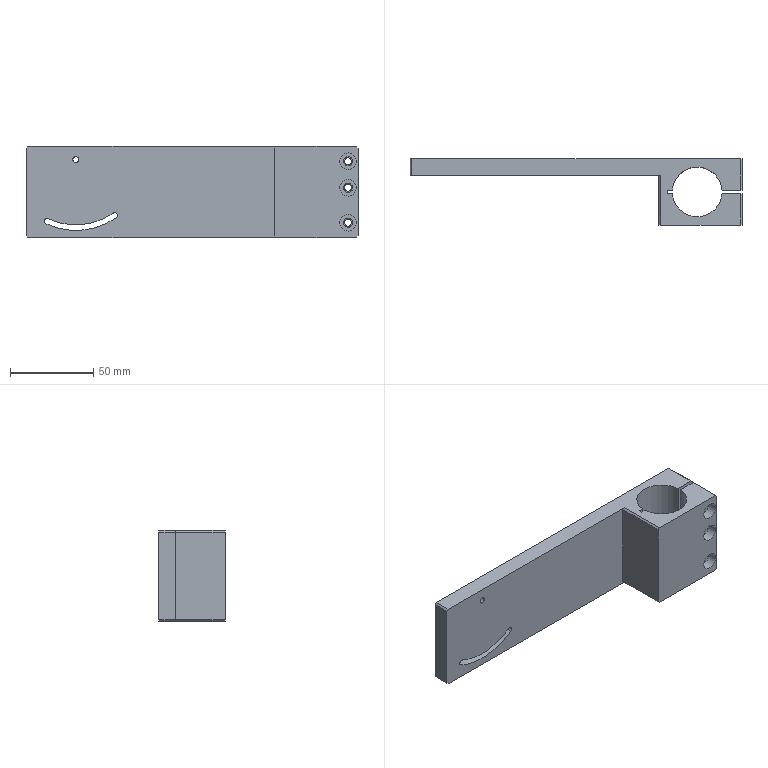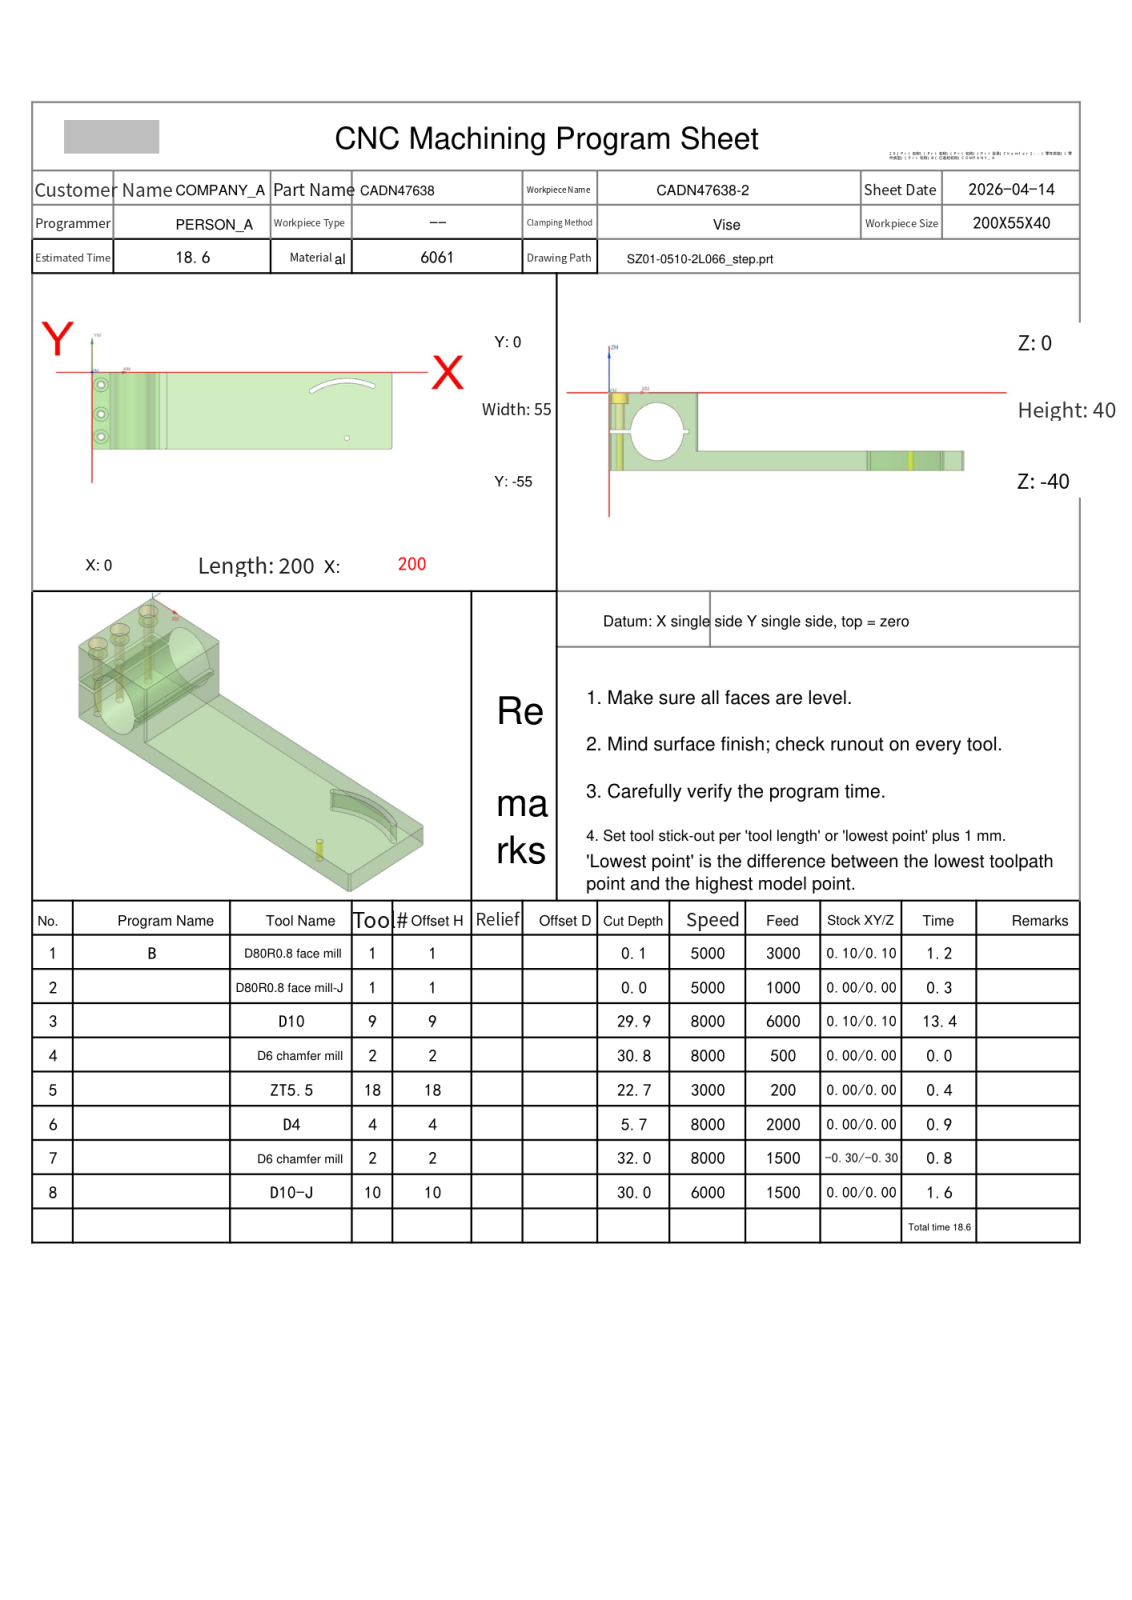NC program | NX | posted by the shop | part box 200 x 40 x 55 mm
Lines 113 to 1145 of 8619:
N3 T09 M06
(D10  D=10. R=0. H=09 ce=0.10 di=0.10)
(MAX_Z=14.8 MIN_Z=-29.9 Time=13.16M)
G00 G90 G54 X202.518 Y7.619 M03 S8000
G43 H09 Z14.8
M08
Z.902
G01 Z-.598 F6000.
X202.583 Y3.347
G02 X202.6 Y1.125 I-147.483 J-2.234
G01 Y-56.112
G02 X202.589 Y-57.94 I-147.5 J0.0
X202.296 Y-58.633 I-1. J.013
G01 X201.322 Y-59.607
G02 X200.616 Y-59.9 I-.707 J.707
G01 X198.47
G02 X197.571 Y-59. I.001 J.9
G01 Y-58.982
G03 X197.6 Y-56.112 I-142.471 J2.87
G01 Y1.124
G03 X197.572 Y3.92 I-142.5 J-.012
X196.573 Y4.9 I-1. J-.02
G01 X190.969
G03 X190.069 Y4. I.001 J-.9
G01 X190.07 Y3.981
G02 X190.1 Y1.124 I-134.97 J-2.869
G01 Y-56.112
G02 X190.071 Y-58.921 I-135. J0.0
X189.071 Y-59.9 I-1. J.021
G01 X183.467
G02 X182.568 Y-59. I.001 J.9
G01 Y-58.98
G03 X182.6 Y-56.112 I-127.468 J2.868
G01 Y1.123
G03 X182.569 Y3.922 I-127.5 J-.01
X181.57 Y4.9 I-1. J-.022
G01 X175.965
G03 X175.066 Y4. I.001 J-.9
G01 Y3.979
G02 X175.1 Y1.122 I-119.966 J-2.867
G01 Y-56.112
G02 X175.067 Y-58.924 I-120. J0.0
X174.068 Y-59.9 I-1. J.024
G01 X168.463
G02 X167.563 Y-59. I.001 J.9
G01 X167.564 Y-58.978
G03 X167.6 Y-56.112 I-112.464 J2.865
G01 Y1.122
G03 X167.565 Y3.925 I-112.5 J-.009
X166.565 Y4.9 I-1. J-.025
G01 X160.96
G03 X160.061 Y4. I.001 J-.9
G01 Y3.976
G02 X160.1 Y1.121 I-104.961 J-2.863
G01 Y-56.112
G02 X160.062 Y-58.927 I-105. J0.0
X159.063 Y-59.9 I-1. J.027
G01 X153.457
G02 X152.558 Y-59. I.001 J.9
G01 Y-58.974
G03 X152.6 Y-56.112 I-97.458 J2.862
G01 Y1.12
G03 X152.559 Y3.929 I-97.5 J-.008
X151.56 Y4.9 I-1. J-.029
G01 X145.954
G03 X145.054 Y4. I.001 J-.9
G01 X145.055 Y3.972
G02 X145.1 Y1.12 I-89.955 J-2.859
G01 Y-56.112
G02 X145.056 Y-58.932 I-90. J0.0
X144.057 Y-59.9 I-1. J.032
G01 X138.45
G02 X137.55 Y-59. I0.0 J.9
G01 X137.551 Y-58.969
G03 X137.6 Y-56.112 I-82.451 J2.857
G01 Y1.119
G03 X137.552 Y3.934 I-82.5 J-.007
X136.553 Y4.9 I-.999 J-.034
G01 X130.945
G03 X130.045 Y4. I.001 J-.9
G01 X130.046 Y3.966
G02 X130.1 Y1.119 I-74.946 J-2.854
G01 Y-56.112
G02 X130.047 Y-58.938 I-75. J0.0
X129.048 Y-59.9 I-.999 J.038
G01 X123.438
G02 X122.539 Y-59. I.001 J.9
G01 X122.54 Y-58.963
G03 X122.6 Y-56.112 I-67.44 J2.85
G01 Y1.118
G03 X122.541 Y3.942 I-67.5 J-.006
X121.542 Y4.9 I-.999 J-.042
G01 X115.931
G03 X115.032 Y4. I.001 J-.9
G01 Y3.958
G02 X115.1 Y1.117 I-59.932 J-2.845
G01 Y-56.112
G02 X115.033 Y-58.948 I-60. J0.0
X114.034 Y-59.9 I-.999 J.048
G01 X108.421
G02 X107.522 Y-59. I.001 J.9
G01 X107.523 Y-58.952
G03 X107.6 Y-56.112 I-52.423 J2.839
G01 Y1.117
G03 X107.523 Y3.954 I-52.5 J-.004
X106.525 Y4.9 I-.999 J-.054
G01 X100.909
G03 X100.009 Y4. I.001 J-.9
G01 X100.011 Y3.944
G02 X100.1 Y1.116 I-44.911 J-2.831
G01 Y-56.112
G02 X100.01 Y-58.964 I-45. J0.0
X99.012 Y-59.9 I-.998 J.064
G01 X93.391
G02 X92.491 Y-59. I.001 J.9
G01 X92.494 Y-58.933
G03 X92.6 Y-56.112 I-37.394 J2.82
G01 Y1.116
G03 X92.49 Y3.977 I-37.5 J-.003
X91.494 Y4.9 I-.997 J-.077
G01 X85.754
G03 X84.955 Y4.1 I.001 J-.8
G01 X84.958 Y4.023
G02 X85.1 Y1.115 I-29.858 J-2.91
G01 Y-56.112
G02 X84.961 Y-58.996 I-30. J0.0
X83.966 Y-59.9 I-.995 J.096
G01 X78.207
G02 X77.408 Y-59.1 I0.0 J.8
G01 X77.414 Y-58.998
G03 X77.6 Y-56.112 I-22.314 J2.885
G01 Y1.114
G03 X77.41 Y4.03 I-22.5 J-.002
X76.419 Y4.9 I-.992 J-.13
G01 X70.493
G03 X69.793 Y4.2 I0.0 J-.7
G01 X69.807 Y4.063
G02 X70.1 Y1.114 I-14.707 J-2.95
G01 Y-56.112
G02 X69.8 Y-59.099 I-15. J0.0
X68.82 Y-59.9 I-.98 J.199
G01 X62.546
G02 X61.946 Y-59.3 I0.0 J.6
X61.995 Y-59.064 I.6 J0.0
G03 X62.6 Y-56.112 I-6.895 J2.952
G01 Y1.112
G03 X61.818 Y4.446 I-7.5 J0.0
X61.101 Y4.985 I-.896 J-.445
G01 X52.197 Y6.591
X52.02 Y6.607
G03 X51.02 Y5.607 I0.0 J-1.
X51.312 Y4.9 I1. J0.0
G01 X55.1 Y1.112
Y-56.112
X51.312 Y-59.9
X48.112 Y-63.1
Z.902
G00 X202.518 Y7.619
Z.304
G01 Z-1.196
X202.583 Y3.347
G02 X202.6 Y1.125 I-147.483 J-2.234
G01 Y-56.112
G02 X202.589 Y-57.94 I-147.5 J0.0
X202.296 Y-58.633 I-1. J.013
G01 X201.322 Y-59.607
G02 X200.616 Y-59.9 I-.707 J.707
G01 X198.47
G02 X197.571 Y-59. I.001 J.9
G01 Y-58.982
G03 X197.6 Y-56.112 I-142.471 J2.87
G01 Y1.124
G03 X197.572 Y3.92 I-142.5 J-.012
X196.573 Y4.9 I-1. J-.02
G01 X190.969
G03 X190.069 Y4. I.001 J-.9
G01 X190.07 Y3.981
G02 X190.1 Y1.124 I-134.97 J-2.869
G01 Y-56.112
G02 X190.071 Y-58.921 I-135. J0.0
X189.071 Y-59.9 I-1. J.021
G01 X183.467
G02 X182.568 Y-59. I.001 J.9
G01 Y-58.98
G03 X182.6 Y-56.112 I-127.468 J2.868
G01 Y1.123
G03 X182.569 Y3.922 I-127.5 J-.01
X181.57 Y4.9 I-1. J-.022
G01 X175.965
G03 X175.066 Y4. I.001 J-.9
G01 Y3.979
G02 X175.1 Y1.122 I-119.966 J-2.867
G01 Y-56.112
G02 X175.067 Y-58.924 I-120. J0.0
X174.068 Y-59.9 I-1. J.024
G01 X168.463
G02 X167.563 Y-59. I.001 J.9
G01 X167.564 Y-58.978
G03 X167.6 Y-56.112 I-112.464 J2.865
G01 Y1.122
G03 X167.565 Y3.925 I-112.5 J-.009
X166.565 Y4.9 I-1. J-.025
G01 X160.96
G03 X160.061 Y4. I.001 J-.9
G01 Y3.976
G02 X160.1 Y1.121 I-104.961 J-2.863
G01 Y-56.112
G02 X160.062 Y-58.927 I-105. J0.0
X159.063 Y-59.9 I-1. J.027
G01 X153.457
G02 X152.558 Y-59. I.001 J.9
G01 Y-58.974
G03 X152.6 Y-56.112 I-97.458 J2.862
G01 Y1.12
G03 X152.559 Y3.929 I-97.5 J-.008
X151.56 Y4.9 I-1. J-.029
G01 X145.954
G03 X145.054 Y4. I.001 J-.9
G01 X145.055 Y3.972
G02 X145.1 Y1.12 I-89.955 J-2.859
G01 Y-56.112
G02 X145.056 Y-58.932 I-90. J0.0
X144.057 Y-59.9 I-1. J.032
G01 X138.45
G02 X137.55 Y-59. I0.0 J.9
G01 X137.551 Y-58.969
G03 X137.6 Y-56.112 I-82.451 J2.857
G01 Y1.119
G03 X137.552 Y3.934 I-82.5 J-.007
X136.553 Y4.9 I-.999 J-.034
G01 X130.945
G03 X130.045 Y4. I.001 J-.9
G01 X130.046 Y3.966
G02 X130.1 Y1.119 I-74.946 J-2.854
G01 Y-56.112
G02 X130.047 Y-58.938 I-75. J0.0
X129.048 Y-59.9 I-.999 J.038
G01 X123.438
G02 X122.539 Y-59. I.001 J.9
G01 X122.54 Y-58.963
G03 X122.6 Y-56.112 I-67.44 J2.85
G01 Y1.118
G03 X122.541 Y3.942 I-67.5 J-.006
X121.542 Y4.9 I-.999 J-.042
G01 X115.931
G03 X115.032 Y4. I.001 J-.9
G01 Y3.958
G02 X115.1 Y1.117 I-59.932 J-2.845
G01 Y-56.112
G02 X115.033 Y-58.948 I-60. J0.0
X114.034 Y-59.9 I-.999 J.048
G01 X108.421
G02 X107.522 Y-59. I.001 J.9
G01 X107.523 Y-58.952
G03 X107.6 Y-56.112 I-52.423 J2.839
G01 Y1.117
G03 X107.523 Y3.954 I-52.5 J-.004
X106.525 Y4.9 I-.999 J-.054
G01 X100.909
G03 X100.009 Y4. I.001 J-.9
G01 X100.011 Y3.944
G02 X100.1 Y1.116 I-44.911 J-2.831
G01 Y-56.112
G02 X100.01 Y-58.964 I-45. J0.0
X99.012 Y-59.9 I-.998 J.064
G01 X93.391
G02 X92.491 Y-59. I.001 J.9
G01 X92.494 Y-58.933
G03 X92.6 Y-56.112 I-37.394 J2.82
G01 Y1.116
G03 X92.49 Y3.977 I-37.5 J-.003
X91.494 Y4.9 I-.997 J-.077
G01 X85.754
G03 X84.955 Y4.1 I.001 J-.8
G01 X84.958 Y4.023
G02 X85.1 Y1.115 I-29.858 J-2.91
G01 Y-56.112
G02 X84.961 Y-58.996 I-30. J0.0
X83.966 Y-59.9 I-.995 J.096
G01 X78.207
G02 X77.408 Y-59.1 I0.0 J.8
G01 X77.414 Y-58.998
G03 X77.6 Y-56.112 I-22.314 J2.885
G01 Y1.114
G03 X77.41 Y4.03 I-22.5 J-.002
X76.419 Y4.9 I-.992 J-.13
G01 X70.493
G03 X69.793 Y4.2 I0.0 J-.7
G01 X69.807 Y4.063
G02 X70.1 Y1.114 I-14.707 J-2.95
G01 Y-56.112
G02 X69.8 Y-59.099 I-15. J0.0
X68.82 Y-59.9 I-.98 J.199
G01 X62.546
G02 X61.946 Y-59.3 I0.0 J.6
X61.995 Y-59.064 I.6 J0.0
G03 X62.6 Y-56.112 I-6.895 J2.952
G01 Y1.112
G03 X61.818 Y4.446 I-7.5 J0.0
X61.101 Y4.985 I-.896 J-.445
G01 X52.197 Y6.591
X52.02 Y6.607
G03 X51.02 Y5.607 I0.0 J-1.
X51.312 Y4.9 I1. J0.0
G01 X55.1 Y1.112
Y-56.112
X51.312 Y-59.9
X48.112 Y-63.1
Z.304
G00 X202.518 Y7.619
Z-.294
G01 Z-1.794
X202.583 Y3.347
G02 X202.6 Y1.125 I-147.483 J-2.234
G01 Y-56.112
G02 X202.589 Y-57.94 I-147.5 J0.0
X202.296 Y-58.633 I-1. J.013
G01 X201.322 Y-59.607
G02 X200.616 Y-59.9 I-.707 J.707
G01 X198.47
G02 X197.571 Y-59. I.001 J.9
G01 Y-58.982
G03 X197.6 Y-56.112 I-142.471 J2.87
G01 Y1.124
G03 X197.572 Y3.92 I-142.5 J-.012
X196.573 Y4.9 I-1. J-.02
G01 X190.969
G03 X190.069 Y4. I.001 J-.9
G01 X190.07 Y3.981
G02 X190.1 Y1.124 I-134.97 J-2.869
G01 Y-56.112
G02 X190.071 Y-58.921 I-135. J0.0
X189.071 Y-59.9 I-1. J.021
G01 X183.467
G02 X182.568 Y-59. I.001 J.9
G01 Y-58.98
G03 X182.6 Y-56.112 I-127.468 J2.868
G01 Y1.123
G03 X182.569 Y3.922 I-127.5 J-.01
X181.57 Y4.9 I-1. J-.022
G01 X175.965
G03 X175.066 Y4. I.001 J-.9
G01 Y3.979
G02 X175.1 Y1.122 I-119.966 J-2.867
G01 Y-56.112
G02 X175.067 Y-58.924 I-120. J0.0
X174.068 Y-59.9 I-1. J.024
G01 X168.463
G02 X167.563 Y-59. I.001 J.9
G01 X167.564 Y-58.978
G03 X167.6 Y-56.112 I-112.464 J2.865
G01 Y1.122
G03 X167.565 Y3.925 I-112.5 J-.009
X166.565 Y4.9 I-1. J-.025
G01 X160.96
G03 X160.061 Y4. I.001 J-.9
G01 Y3.976
G02 X160.1 Y1.121 I-104.961 J-2.863
G01 Y-56.112
G02 X160.062 Y-58.927 I-105. J0.0
X159.063 Y-59.9 I-1. J.027
G01 X153.457
G02 X152.558 Y-59. I.001 J.9
G01 Y-58.974
G03 X152.6 Y-56.112 I-97.458 J2.862
G01 Y1.12
G03 X152.559 Y3.929 I-97.5 J-.008
X151.56 Y4.9 I-1. J-.029
G01 X145.954
G03 X145.054 Y4. I.001 J-.9
G01 X145.055 Y3.972
G02 X145.1 Y1.12 I-89.955 J-2.859
G01 Y-56.112
G02 X145.056 Y-58.932 I-90. J0.0
X144.057 Y-59.9 I-1. J.032
G01 X138.45
G02 X137.55 Y-59. I0.0 J.9
G01 X137.551 Y-58.969
G03 X137.6 Y-56.112 I-82.451 J2.857
G01 Y1.119
G03 X137.552 Y3.934 I-82.5 J-.007
X136.553 Y4.9 I-.999 J-.034
G01 X130.945
G03 X130.045 Y4. I.001 J-.9
G01 X130.046 Y3.966
G02 X130.1 Y1.119 I-74.946 J-2.854
G01 Y-56.112
G02 X130.047 Y-58.938 I-75. J0.0
X129.048 Y-59.9 I-.999 J.038
G01 X123.438
G02 X122.539 Y-59. I.001 J.9
G01 X122.54 Y-58.963
G03 X122.6 Y-56.112 I-67.44 J2.85
G01 Y1.118
G03 X122.541 Y3.942 I-67.5 J-.006
X121.542 Y4.9 I-.999 J-.042
G01 X115.931
G03 X115.032 Y4. I.001 J-.9
G01 Y3.958
G02 X115.1 Y1.117 I-59.932 J-2.845
G01 Y-56.112
G02 X115.033 Y-58.948 I-60. J0.0
X114.034 Y-59.9 I-.999 J.048
G01 X108.421
G02 X107.522 Y-59. I.001 J.9
G01 X107.523 Y-58.952
G03 X107.6 Y-56.112 I-52.423 J2.839
G01 Y1.117
G03 X107.523 Y3.954 I-52.5 J-.004
X106.525 Y4.9 I-.999 J-.054
G01 X100.909
G03 X100.009 Y4. I.001 J-.9
G01 X100.011 Y3.944
G02 X100.1 Y1.116 I-44.911 J-2.831
G01 Y-56.112
G02 X100.01 Y-58.964 I-45. J0.0
X99.012 Y-59.9 I-.998 J.064
G01 X93.391
G02 X92.491 Y-59. I.001 J.9
G01 X92.494 Y-58.933
G03 X92.6 Y-56.112 I-37.394 J2.82
G01 Y1.116
G03 X92.49 Y3.977 I-37.5 J-.003
X91.494 Y4.9 I-.997 J-.077
G01 X85.754
G03 X84.955 Y4.1 I.001 J-.8
G01 X84.958 Y4.023
G02 X85.1 Y1.115 I-29.858 J-2.91
G01 Y-56.112
G02 X84.961 Y-58.996 I-30. J0.0
X83.966 Y-59.9 I-.995 J.096
G01 X78.207
G02 X77.408 Y-59.1 I0.0 J.8
G01 X77.414 Y-58.998
G03 X77.6 Y-56.112 I-22.314 J2.885
G01 Y1.114
G03 X77.41 Y4.03 I-22.5 J-.002
X76.419 Y4.9 I-.992 J-.13
G01 X70.493
G03 X69.793 Y4.2 I0.0 J-.7
G01 X69.807 Y4.063
G02 X70.1 Y1.114 I-14.707 J-2.95
G01 Y-56.112
G02 X69.8 Y-59.099 I-15. J0.0
X68.82 Y-59.9 I-.98 J.199
G01 X62.546
G02 X61.946 Y-59.3 I0.0 J.6
X61.995 Y-59.064 I.6 J0.0
G03 X62.6 Y-56.112 I-6.895 J2.952
G01 Y1.112
G03 X61.818 Y4.446 I-7.5 J0.0
X61.101 Y4.985 I-.896 J-.445
G01 X52.197 Y6.591
X52.02 Y6.607
G03 X51.02 Y5.607 I0.0 J-1.
X51.312 Y4.9 I1. J0.0
G01 X55.1 Y1.112
Y-56.112
X51.312 Y-59.9
X48.112 Y-63.1
Z-.294
G00 X202.518 Y7.619
Z-.892
G01 Z-2.392
X202.583 Y3.347
G02 X202.6 Y1.125 I-147.483 J-2.234
G01 Y-56.112
G02 X202.589 Y-57.94 I-147.5 J0.0
X202.296 Y-58.633 I-1. J.013
G01 X201.322 Y-59.607
G02 X200.616 Y-59.9 I-.707 J.707
G01 X198.47
G02 X197.571 Y-59. I.001 J.9
G01 Y-58.982
G03 X197.6 Y-56.112 I-142.471 J2.87
G01 Y1.124
G03 X197.572 Y3.92 I-142.5 J-.012
X196.573 Y4.9 I-1. J-.02
G01 X190.969
G03 X190.069 Y4. I.001 J-.9
G01 X190.07 Y3.981
G02 X190.1 Y1.124 I-134.97 J-2.869
G01 Y-56.112
G02 X190.071 Y-58.921 I-135. J0.0
X189.071 Y-59.9 I-1. J.021
G01 X183.467
G02 X182.568 Y-59. I.001 J.9
G01 Y-58.98
G03 X182.6 Y-56.112 I-127.468 J2.868
G01 Y1.123
G03 X182.569 Y3.922 I-127.5 J-.01
X181.57 Y4.9 I-1. J-.022
G01 X175.965
G03 X175.066 Y4. I.001 J-.9
G01 Y3.979
G02 X175.1 Y1.122 I-119.966 J-2.867
G01 Y-56.112
G02 X175.067 Y-58.924 I-120. J0.0
X174.068 Y-59.9 I-1. J.024
G01 X168.463
G02 X167.563 Y-59. I.001 J.9
G01 X167.564 Y-58.978
G03 X167.6 Y-56.112 I-112.464 J2.865
G01 Y1.122
G03 X167.565 Y3.925 I-112.5 J-.009
X166.565 Y4.9 I-1. J-.025
G01 X160.96
G03 X160.061 Y4. I.001 J-.9
G01 Y3.976
G02 X160.1 Y1.121 I-104.961 J-2.863
G01 Y-56.112
G02 X160.062 Y-58.927 I-105. J0.0
X159.063 Y-59.9 I-1. J.027
G01 X153.457
G02 X152.558 Y-59. I.001 J.9
G01 Y-58.974
G03 X152.6 Y-56.112 I-97.458 J2.862
G01 Y1.12
G03 X152.559 Y3.929 I-97.5 J-.008
X151.56 Y4.9 I-1. J-.029
G01 X145.954
G03 X145.054 Y4. I.001 J-.9
G01 X145.055 Y3.972
G02 X145.1 Y1.12 I-89.955 J-2.859
G01 Y-56.112
G02 X145.056 Y-58.932 I-90. J0.0
X144.057 Y-59.9 I-1. J.032
G01 X138.45
G02 X137.55 Y-59. I0.0 J.9
G01 X137.551 Y-58.969
G03 X137.6 Y-56.112 I-82.451 J2.857
G01 Y1.119
G03 X137.552 Y3.934 I-82.5 J-.007
X136.553 Y4.9 I-.999 J-.034
G01 X130.945
G03 X130.045 Y4. I.001 J-.9
G01 X130.046 Y3.966
G02 X130.1 Y1.119 I-74.946 J-2.854
G01 Y-56.112
G02 X130.047 Y-58.938 I-75. J0.0
X129.048 Y-59.9 I-.999 J.038
G01 X123.438
G02 X122.539 Y-59. I.001 J.9
G01 X122.54 Y-58.963
G03 X122.6 Y-56.112 I-67.44 J2.85
G01 Y1.118
G03 X122.541 Y3.942 I-67.5 J-.006
X121.542 Y4.9 I-.999 J-.042
G01 X115.931
G03 X115.032 Y4. I.001 J-.9
G01 Y3.958
G02 X115.1 Y1.117 I-59.932 J-2.845
G01 Y-56.112
G02 X115.033 Y-58.948 I-60. J0.0
X114.034 Y-59.9 I-.999 J.048
G01 X108.421
G02 X107.522 Y-59. I.001 J.9
G01 X107.523 Y-58.952
G03 X107.6 Y-56.112 I-52.423 J2.839
G01 Y1.117
G03 X107.523 Y3.954 I-52.5 J-.004
X106.525 Y4.9 I-.999 J-.054
G01 X100.909
G03 X100.009 Y4. I.001 J-.9
G01 X100.011 Y3.944
G02 X100.1 Y1.116 I-44.911 J-2.831
G01 Y-56.112
G02 X100.01 Y-58.964 I-45. J0.0
X99.012 Y-59.9 I-.998 J.064
G01 X93.391
G02 X92.491 Y-59. I.001 J.9
G01 X92.494 Y-58.933
G03 X92.6 Y-56.112 I-37.394 J2.82
G01 Y1.116
G03 X92.49 Y3.977 I-37.5 J-.003
X91.494 Y4.9 I-.997 J-.077
G01 X85.754
G03 X84.955 Y4.1 I.001 J-.8
G01 X84.958 Y4.023
G02 X85.1 Y1.115 I-29.858 J-2.91
G01 Y-56.112
G02 X84.961 Y-58.996 I-30. J0.0
X83.966 Y-59.9 I-.995 J.096
G01 X78.207
G02 X77.408 Y-59.1 I0.0 J.8
G01 X77.414 Y-58.998
G03 X77.6 Y-56.112 I-22.314 J2.885
G01 Y1.114
G03 X77.41 Y4.03 I-22.5 J-.002
X76.419 Y4.9 I-.992 J-.13
G01 X70.493
G03 X69.793 Y4.2 I0.0 J-.7
G01 X69.807 Y4.063
G02 X70.1 Y1.114 I-14.707 J-2.95
G01 Y-56.112
G02 X69.8 Y-59.099 I-15. J0.0
X68.82 Y-59.9 I-.98 J.199
G01 X62.546
G02 X61.946 Y-59.3 I0.0 J.6
X61.995 Y-59.064 I.6 J0.0
G03 X62.6 Y-56.112 I-6.895 J2.952
G01 Y1.112
G03 X61.818 Y4.446 I-7.5 J0.0
X61.101 Y4.985 I-.896 J-.445
G01 X52.197 Y6.591
X52.02 Y6.607
G03 X51.02 Y5.607 I0.0 J-1.
X51.312 Y4.9 I1. J0.0
G01 X55.1 Y1.112
Y-56.112
X51.312 Y-59.9
X48.112 Y-63.1
Z-.892
G00 X202.518 Y7.619
Z-1.49
G01 Z-2.99
X202.583 Y3.347
G02 X202.6 Y1.125 I-147.483 J-2.234
G01 Y-56.112
G02 X202.589 Y-57.94 I-147.5 J0.0
X202.296 Y-58.633 I-1. J.013
G01 X201.322 Y-59.607
G02 X200.616 Y-59.9 I-.707 J.707
G01 X198.47
G02 X197.571 Y-59. I.001 J.9
G01 Y-58.982
G03 X197.6 Y-56.112 I-142.471 J2.87
G01 Y1.124
G03 X197.572 Y3.92 I-142.5 J-.012
X196.573 Y4.9 I-1. J-.02
G01 X190.969
G03 X190.069 Y4. I.001 J-.9
G01 X190.07 Y3.981
G02 X190.1 Y1.124 I-134.97 J-2.869
G01 Y-56.112
G02 X190.071 Y-58.921 I-135. J0.0
X189.071 Y-59.9 I-1. J.021
G01 X183.467
G02 X182.568 Y-59. I.001 J.9
G01 Y-58.98
G03 X182.6 Y-56.112 I-127.468 J2.868
G01 Y1.123
G03 X182.569 Y3.922 I-127.5 J-.01
X181.57 Y4.9 I-1. J-.022
G01 X175.965
G03 X175.066 Y4. I.001 J-.9
G01 Y3.979
G02 X175.1 Y1.122 I-119.966 J-2.867
G01 Y-56.112
G02 X175.067 Y-58.924 I-120. J0.0
X174.068 Y-59.9 I-1. J.024
G01 X168.463
G02 X167.563 Y-59. I.001 J.9
G01 X167.564 Y-58.978
G03 X167.6 Y-56.112 I-112.464 J2.865
G01 Y1.122
G03 X167.565 Y3.925 I-112.5 J-.009
X166.565 Y4.9 I-1. J-.025
G01 X160.96
G03 X160.061 Y4. I.001 J-.9
G01 Y3.976
G02 X160.1 Y1.121 I-104.961 J-2.863
G01 Y-56.112
G02 X160.062 Y-58.927 I-105. J0.0
X159.063 Y-59.9 I-1. J.027
G01 X153.457
G02 X152.558 Y-59. I.001 J.9
G01 Y-58.974
G03 X152.6 Y-56.112 I-97.458 J2.862
G01 Y1.12
G03 X152.559 Y3.929 I-97.5 J-.008
X151.56 Y4.9 I-1. J-.029
G01 X145.954
G03 X145.054 Y4. I.001 J-.9
G01 X145.055 Y3.972
G02 X145.1 Y1.12 I-89.955 J-2.859
G01 Y-56.112
G02 X145.056 Y-58.932 I-90. J0.0
X144.057 Y-59.9 I-1. J.032
G01 X138.45
G02 X137.55 Y-59. I0.0 J.9
G01 X137.551 Y-58.969
G03 X137.6 Y-56.112 I-82.451 J2.857
G01 Y1.119
G03 X137.552 Y3.934 I-82.5 J-.007
X136.553 Y4.9 I-.999 J-.034
G01 X130.945
G03 X130.045 Y4. I.001 J-.9
G01 X130.046 Y3.966
G02 X130.1 Y1.119 I-74.946 J-2.854
G01 Y-56.112
G02 X130.047 Y-58.938 I-75. J0.0
X129.048 Y-59.9 I-.999 J.038
G01 X123.438
G02 X122.539 Y-59. I.001 J.9
G01 X122.54 Y-58.963
G03 X122.6 Y-56.112 I-67.44 J2.85
G01 Y1.118
G03 X122.541 Y3.942 I-67.5 J-.006
X121.542 Y4.9 I-.999 J-.042
G01 X115.931
G03 X115.032 Y4. I.001 J-.9
G01 Y3.958
G02 X115.1 Y1.117 I-59.932 J-2.845
G01 Y-56.112
G02 X115.033 Y-58.948 I-60. J0.0
X114.034 Y-59.9 I-.999 J.048
G01 X108.421
G02 X107.522 Y-59. I.001 J.9
G01 X107.523 Y-58.952
G03 X107.6 Y-56.112 I-52.423 J2.839
G01 Y1.117
G03 X107.523 Y3.954 I-52.5 J-.004
X106.525 Y4.9 I-.999 J-.054
G01 X100.909
G03 X100.009 Y4. I.001 J-.9
G01 X100.011 Y3.944
G02 X100.1 Y1.116 I-44.911 J-2.831
G01 Y-56.112
G02 X100.01 Y-58.964 I-45. J0.0
X99.012 Y-59.9 I-.998 J.064
G01 X93.391
G02 X92.491 Y-59. I.001 J.9
G01 X92.494 Y-58.933
G03 X92.6 Y-56.112 I-37.394 J2.82
G01 Y1.116
G03 X92.49 Y3.977 I-37.5 J-.003
X91.494 Y4.9 I-.997 J-.077
G01 X85.754
G03 X84.955 Y4.1 I.001 J-.8
G01 X84.958 Y4.023
G02 X85.1 Y1.115 I-29.858 J-2.91
G01 Y-56.112
G02 X84.961 Y-58.996 I-30. J0.0
X83.966 Y-59.9 I-.995 J.096
G01 X78.207
G02 X77.408 Y-59.1 I0.0 J.8
G01 X77.414 Y-58.998
G03 X77.6 Y-56.112 I-22.314 J2.885
G01 Y1.114
G03 X77.41 Y4.03 I-22.5 J-.002
X76.419 Y4.9 I-.992 J-.13
G01 X70.493
G03 X69.793 Y4.2 I0.0 J-.7
G01 X69.807 Y4.063
G02 X70.1 Y1.114 I-14.707 J-2.95
G01 Y-56.112
G02 X69.8 Y-59.099 I-15. J0.0
X68.82 Y-59.9 I-.98 J.199
G01 X62.546
G02 X61.946 Y-59.3 I0.0 J.6
X61.995 Y-59.064 I.6 J0.0
G03 X62.6 Y-56.112 I-6.895 J2.952
G01 Y1.112
G03 X61.818 Y4.446 I-7.5 J0.0
X61.101 Y4.985 I-.896 J-.445
G01 X52.197 Y6.591
X52.02 Y6.607
G03 X51.02 Y5.607 I0.0 J-1.
X51.312 Y4.9 I1. J0.0
G01 X55.1 Y1.112
Y-56.112
X51.312 Y-59.9
X48.112 Y-63.1
Z-1.49
G00 X202.518 Y7.619
Z-2.088
G01 Z-3.588
X202.583 Y3.347
G02 X202.6 Y1.125 I-147.483 J-2.234
G01 Y-56.112
G02 X202.589 Y-57.94 I-147.5 J0.0
X202.296 Y-58.633 I-1. J.013
G01 X201.322 Y-59.607
G02 X200.616 Y-59.9 I-.707 J.707
G01 X198.47
G02 X197.571 Y-59. I.001 J.9
G01 Y-58.982
G03 X197.6 Y-56.112 I-142.471 J2.87
G01 Y1.124
G03 X197.572 Y3.92 I-142.5 J-.012
X196.573 Y4.9 I-1. J-.02
G01 X190.969
G03 X190.069 Y4. I.001 J-.9
G01 X190.07 Y3.981
G02 X190.1 Y1.124 I-134.97 J-2.869
G01 Y-56.112
G02 X190.071 Y-58.921 I-135. J0.0
X189.071 Y-59.9 I-1. J.021
G01 X183.467
G02 X182.568 Y-59. I.001 J.9
G01 Y-58.98
G03 X182.6 Y-56.112 I-127.468 J2.868
G01 Y1.123
G03 X182.569 Y3.922 I-127.5 J-.01
X181.57 Y4.9 I-1. J-.022
G01 X175.965
G03 X175.066 Y4. I.001 J-.9
G01 Y3.979
G02 X175.1 Y1.122 I-119.966 J-2.867
G01 Y-56.112
G02 X175.067 Y-58.924 I-120. J0.0
X174.068 Y-59.9 I-1. J.024
G01 X168.463
G02 X167.563 Y-59. I.001 J.9
G01 X167.564 Y-58.978
G03 X167.6 Y-56.112 I-112.464 J2.865
G01 Y1.122
G03 X167.565 Y3.925 I-112.5 J-.009
X166.565 Y4.9 I-1. J-.025
G01 X160.96
G03 X160.061 Y4. I.001 J-.9
G01 Y3.976
G02 X160.1 Y1.121 I-104.961 J-2.863
G01 Y-56.112
G02 X160.062 Y-58.927 I-105. J0.0
X159.063 Y-59.9 I-1. J.027
G01 X153.457
G02 X152.558 Y-59. I.001 J.9
G01 Y-58.974
G03 X152.6 Y-56.112 I-97.458 J2.862
G01 Y1.12
G03 X152.559 Y3.929 I-97.5 J-.008
X151.56 Y4.9 I-1. J-.029
G01 X145.954
G03 X145.054 Y4. I.001 J-.9
G01 X145.055 Y3.972
G02 X145.1 Y1.12 I-89.955 J-2.859
G01 Y-56.112
G02 X145.056 Y-58.932 I-90. J0.0
X144.057 Y-59.9 I-1. J.032
G01 X138.45
G02 X137.55 Y-59. I0.0 J.9
G01 X137.551 Y-58.969
G03 X137.6 Y-56.112 I-82.451 J2.857
G01 Y1.119
G03 X137.552 Y3.934 I-82.5 J-.007
X136.553 Y4.9 I-.999 J-.034
G01 X130.945
G03 X130.045 Y4. I.001 J-.9
G01 X130.046 Y3.966
G02 X130.1 Y1.119 I-74.946 J-2.854
G01 Y-56.112
G02 X130.047 Y-58.938 I-75. J0.0
X129.048 Y-59.9 I-.999 J.038
G01 X123.438
G02 X122.539 Y-59. I.001 J.9
G01 X122.54 Y-58.963
G03 X122.6 Y-56.112 I-67.44 J2.85
G01 Y1.118
G03 X122.541 Y3.942 I-67.5 J-.006
X121.542 Y4.9 I-.999 J-.042
G01 X115.931
G03 X115.032 Y4. I.001 J-.9
G01 Y3.958
G02 X115.1 Y1.117 I-59.932 J-2.845
G01 Y-56.112
G02 X115.033 Y-58.948 I-60. J0.0
X114.034 Y-59.9 I-.999 J.048
G01 X108.421
G02 X107.522 Y-59. I.001 J.9
G01 X107.523 Y-58.952
G03 X107.6 Y-56.112 I-52.423 J2.839
G01 Y1.117
G03 X107.523 Y3.954 I-52.5 J-.004
X106.525 Y4.9 I-.999 J-.054
G01 X100.909
G03 X100.009 Y4. I.001 J-.9
G01 X100.011 Y3.944
G02 X100.1 Y1.116 I-44.911 J-2.831
G01 Y-56.112
G02 X100.01 Y-58.964 I-45. J0.0
X99.012 Y-59.9 I-.998 J.064
G01 X93.391
G02 X92.491 Y-59. I.001 J.9
G01 X92.494 Y-58.933
G03 X92.6 Y-56.112 I-37.394 J2.82
G01 Y1.116
G03 X92.49 Y3.977 I-37.5 J-.003
X91.494 Y4.9 I-.997 J-.077
G01 X85.754
G03 X84.955 Y4.1 I.001 J-.8
G01 X84.958 Y4.023
G02 X85.1 Y1.115 I-29.858 J-2.91
G01 Y-56.112
G02 X84.961 Y-58.996 I-30. J0.0
X83.966 Y-59.9 I-.995 J.096
G01 X78.207
G02 X77.408 Y-59.1 I0.0 J.8
G01 X77.414 Y-58.998
G03 X77.6 Y-56.112 I-22.314 J2.885
G01 Y1.114
G03 X77.41 Y4.03 I-22.5 J-.002
X76.419 Y4.9 I-.992 J-.13
G01 X70.493
G03 X69.793 Y4.2 I0.0 J-.7
G01 X69.807 Y4.063
G02 X70.1 Y1.114 I-14.707 J-2.95
G01 Y-56.112
G02 X69.8 Y-59.099 I-15. J0.0
X68.82 Y-59.9 I-.98 J.199
G01 X62.546
G02 X61.946 Y-59.3 I0.0 J.6
X61.995 Y-59.064 I.6 J0.0
G03 X62.6 Y-56.112 I-6.895 J2.952
G01 Y1.112
G03 X61.818 Y4.446 I-7.5 J0.0
X61.101 Y4.985 I-.896 J-.445
G01 X52.197 Y6.591
X52.02 Y6.607
G03 X51.02 Y5.607 I0.0 J-1.
X51.312 Y4.9 I1. J0.0
G01 X55.1 Y1.112
Y-56.112
X51.312 Y-59.9
X48.112 Y-63.1
Z-2.088
G00 X202.518 Y7.619
Z-2.686
G01 Z-4.186
X202.583 Y3.347
G02 X202.6 Y1.125 I-147.483 J-2.234
G01 Y-56.112
G02 X202.589 Y-57.94 I-147.5 J0.0
X202.296 Y-58.633 I-1. J.013
G01 X201.322 Y-59.607
G02 X200.616 Y-59.9 I-.707 J.707
G01 X198.47
G02 X197.571 Y-59. I.001 J.9
G01 Y-58.982
G03 X197.6 Y-56.112 I-142.471 J2.87
G01 Y1.124
G03 X197.572 Y3.92 I-142.5 J-.012
X196.573 Y4.9 I-1. J-.02
G01 X190.969
G03 X190.069 Y4. I.001 J-.9
G01 X190.07 Y3.981
G02 X190.1 Y1.124 I-134.97 J-2.869
G01 Y-56.112
G02 X190.071 Y-58.921 I-135. J0.0
X189.071 Y-59.9 I-1. J.021
G01 X183.467
G02 X182.568 Y-59. I.001 J.9
G01 Y-58.98
G03 X182.6 Y-56.112 I-127.468 J2.868
G01 Y1.123
G03 X182.569 Y3.922 I-127.5 J-.01
X181.57 Y4.9 I-1. J-.022
G01 X175.965
G03 X175.066 Y4. I.001 J-.9
G01 Y3.979
G02 X175.1 Y1.122 I-119.966 J-2.867
G01 Y-56.112
G02 X175.067 Y-58.924 I-120. J0.0
X174.068 Y-59.9 I-1. J.024
G01 X168.463
G02 X167.563 Y-59. I.001 J.9
G01 X167.564 Y-58.978
G03 X167.6 Y-56.112 I-112.464 J2.865
G01 Y1.122
G03 X167.565 Y3.925 I-112.5 J-.009
X166.565 Y4.9 I-1. J-.025
G01 X160.96
G03 X160.061 Y4. I.001 J-.9
G01 Y3.976
G02 X160.1 Y1.121 I-104.961 J-2.863
G01 Y-56.112
G02 X160.062 Y-58.927 I-105. J0.0
X159.063 Y-59.9 I-1. J.027
G01 X153.457
G02 X152.558 Y-59. I.001 J.9
G01 Y-58.974
G03 X152.6 Y-56.112 I-97.458 J2.862
G01 Y1.12
G03 X152.559 Y3.929 I-97.5 J-.008
X151.56 Y4.9 I-1. J-.029
G01 X145.954
G03 X145.054 Y4. I.001 J-.9
G01 X145.055 Y3.972
G02 X145.1 Y1.12 I-89.955 J-2.859
G01 Y-56.112
G02 X145.056 Y-58.932 I-90. J0.0
X144.057 Y-59.9 I-1. J.032
G01 X138.45
G02 X137.55 Y-59. I0.0 J.9
G01 X137.551 Y-58.969
G03 X137.6 Y-56.112 I-82.451 J2.857
G01 Y1.119
G03 X137.552 Y3.934 I-82.5 J-.007
X136.553 Y4.9 I-.999 J-.034
G01 X130.945
G03 X130.045 Y4. I.001 J-.9
G01 X130.046 Y3.966
G02 X130.1 Y1.119 I-74.946 J-2.854
G01 Y-56.112
G02 X130.047 Y-58.938 I-75. J0.0
X129.048 Y-59.9 I-.999 J.038
G01 X123.438
G02 X122.539 Y-59. I.001 J.9
G01 X122.54 Y-58.963
G03 X122.6 Y-56.112 I-67.44 J2.85
G01 Y1.118
G03 X122.541 Y3.942 I-67.5 J-.006
X121.542 Y4.9 I-.999 J-.042
G01 X115.931
G03 X115.032 Y4. I.001 J-.9
G01 Y3.958
G02 X115.1 Y1.117 I-59.932 J-2.845
G01 Y-56.112
G02 X115.033 Y-58.948 I-60. J0.0
X114.034 Y-59.9 I-.999 J.048
G01 X108.421
G02 X107.522 Y-59. I.001 J.9
G01 X107.523 Y-58.952
G03 X107.6 Y-56.112 I-52.423 J2.839
G01 Y1.117
G03 X107.523 Y3.954 I-52.5 J-.004
X106.525 Y4.9 I-.999 J-.054
G01 X100.909
G03 X100.009 Y4. I.001 J-.9
G01 X100.011 Y3.944
G02 X100.1 Y1.116 I-44.911 J-2.831
G01 Y-56.112
G02 X100.01 Y-58.964 I-45. J0.0
X99.012 Y-59.9 I-.998 J.064
G01 X93.391
G02 X92.491 Y-59. I.001 J.9
G01 X92.494 Y-58.933
G03 X92.6 Y-56.112 I-37.394 J2.82
G01 Y1.116
G03 X92.49 Y3.977 I-37.5 J-.003
X91.494 Y4.9 I-.997 J-.077
G01 X85.754